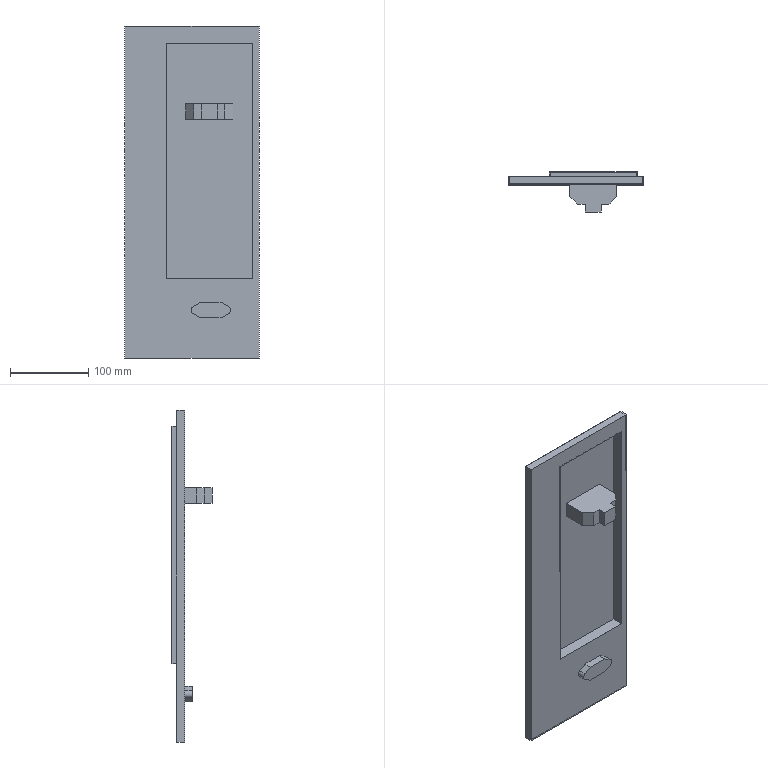Part | STEP file | Computer chassis rear plate_RR | 1 solid | 41 faces | box 172 x 51 x 423 mm | volume 154052 mm3 | plane 39 | cylinder 2 | commonest cylinder face diameters 10.446 x2